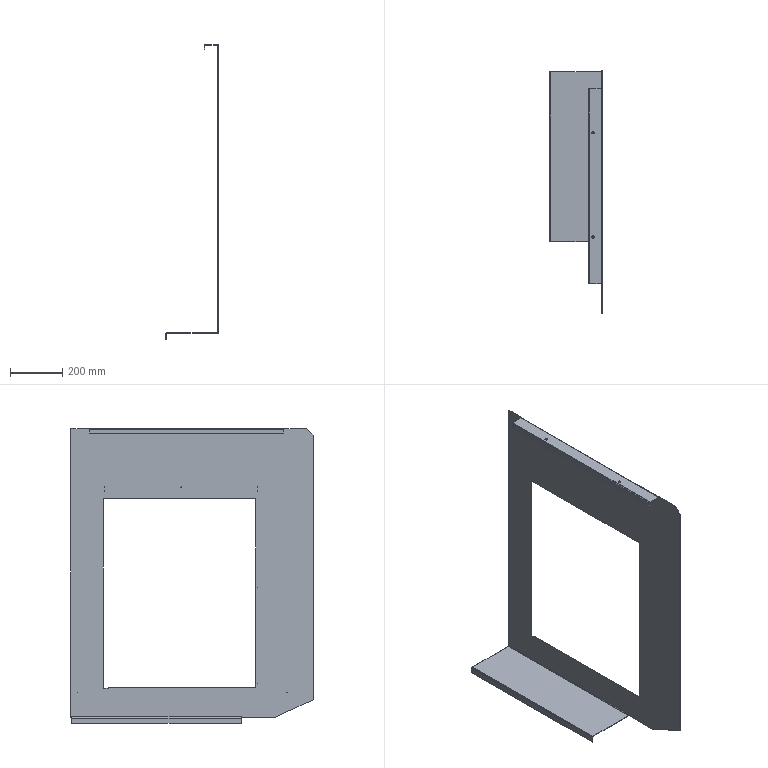Part | NX | features solid 2 | 1 solid | 69 faces | box 203 x 930 x 1133 mm | volume 1592044 mm3 | plane 39 | cylinder 30 | commonest cylinder face diameters 1 x18 4 x4 8 x4 9.2 x4